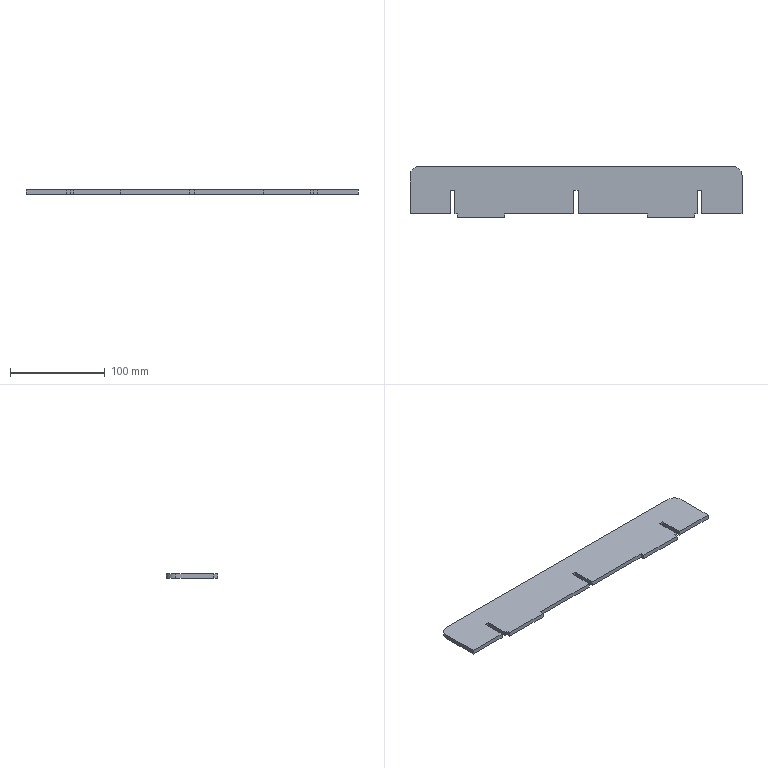Part | SolidWorks | features FlatPattern 1, SMBaseFlange 1, SheetMetal 1 | 1 solid | 28 faces | box 350 x 54 x 4.5 mm | volume 78838 mm3 | plane 26 | cylinder 2 | commonest cylinder face diameters 20 x2
STEP:
#1=CARTESIAN_POINT('',(-308.5,289.731,0.));
#2=VERTEX_POINT('',#1);
#3=CARTESIAN_POINT('',(-308.5,249.731,0.));
#4=VERTEX_POINT('',#3);
#5=CARTESIAN_POINT('',(-308.5,249.731,0.));
#6=DIRECTION('',(0.,-1.,0.));
#7=VECTOR('',#6,1000.);
#8=LINE('',#5,#7);
#9=EDGE_CURVE('',#2,#4,#8,.T.);
#10=ORIENTED_EDGE('',*,*,#9,.F.);
#11=CARTESIAN_POINT('',(-308.5,289.731,-4.5));
#12=VERTEX_POINT('',#11);
#13=CARTESIAN_POINT('',(-308.5,289.731,-4.5));
#14=DIRECTION('',(0.,0.,1.));
#15=VECTOR('',#14,1000.);
#16=LINE('',#13,#15);
#17=EDGE_CURVE('',#12,#2,#16,.T.);
#18=ORIENTED_EDGE('',*,*,#17,.F.);
#19=CARTESIAN_POINT('',(-308.5,249.731,-4.5));
#20=VERTEX_POINT('',#19);
#21=CARTESIAN_POINT('',(-308.5,249.731,-4.5));
#22=DIRECTION('',(0.,-1.,0.));
#23=VECTOR('',#22,1000.);
#24=LINE('',#21,#23);
#25=EDGE_CURVE('',#12,#20,#24,.T.);
#26=ORIENTED_EDGE('',*,*,#25,.T.);
#27=CARTESIAN_POINT('',(-308.5,249.731,-4.5));
#28=DIRECTION('',(0.,0.,1.));
#29=VECTOR('',#28,1000.);
#30=LINE('',#27,#29);
#31=EDGE_CURVE('',#20,#4,#30,.T.);
#32=ORIENTED_EDGE('',*,*,#31,.T.);
#33=EDGE_LOOP('',(#10,#18,#26,#32));
#34=FACE_OUTER_BOUND('',#33,.T.);
#35=CARTESIAN_POINT('',(-308.5,249.731,-4.5));
#36=DIRECTION('',(-1.,0.,0.));
#37=DIRECTION('',(0.,0.,1.));
#38=AXIS2_PLACEMENT_3D('',#35,#36,#37);
#39=PLANE('',#38);
#40=ADVANCED_FACE('',(#34),#39,.T.);
#41=CARTESIAN_POINT('',(-298.5,299.731,0.));
#42=VERTEX_POINT('',#41);
#43=CARTESIAN_POINT('',(-298.5,289.731,0.));
#44=DIRECTION('',(0.,0.,1.));
#45=DIRECTION('',(-1.,0.,0.));
#46=AXIS2_PLACEMENT_3D('',#43,#44,#45);
#47=CIRCLE('',#46,10.);
#48=EDGE_CURVE('',#42,#2,#47,.T.);
#49=ORIENTED_EDGE('',*,*,#48,.F.);
#50=CARTESIAN_POINT('',(-298.5,299.731,-4.5));
#51=VERTEX_POINT('',#50);
#52=CARTESIAN_POINT('',(-298.5,299.731,-4.5));
#53=DIRECTION('',(0.,0.,1.));
#54=VECTOR('',#53,1000.);
#55=LINE('',#52,#54);
#56=EDGE_CURVE('',#51,#42,#55,.T.);
#57=ORIENTED_EDGE('',*,*,#56,.F.);
#58=CARTESIAN_POINT('',(-298.5,289.731,-4.5));
#59=DIRECTION('',(0.,0.,1.));
#60=DIRECTION('',(-1.,0.,0.));
#61=AXIS2_PLACEMENT_3D('',#58,#59,#60);
#62=CIRCLE('',#61,10.);
#63=EDGE_CURVE('',#51,#12,#62,.T.);
#64=ORIENTED_EDGE('',*,*,#63,.T.);
#65=ORIENTED_EDGE('',*,*,#17,.T.);
#66=EDGE_LOOP('',(#49,#57,#64,#65));
#67=FACE_OUTER_BOUND('',#66,.T.);
#68=CARTESIAN_POINT('',(-298.5,289.731,-4.5));
#69=DIRECTION('',(0.,0.,1.));
#70=DIRECTION('',(1.,0.,0.));
#71=AXIS2_PLACEMENT_3D('',#68,#69,#70);
#72=CYLINDRICAL_SURFACE('',#71,10.);
#73=ADVANCED_FACE('',(#67),#72,.T.);
#74=CARTESIAN_POINT('',(31.5,299.731,0.));
#75=VERTEX_POINT('',#74);
#76=CARTESIAN_POINT('',(-298.5,299.731,0.));
#77=DIRECTION('',(-1.,0.,0.));
#78=VECTOR('',#77,1000.);
#79=LINE('',#76,#78);
#80=EDGE_CURVE('',#75,#42,#79,.T.);
#81=ORIENTED_EDGE('',*,*,#80,.F.);
#82=CARTESIAN_POINT('',(31.5,299.731,-4.5));
#83=VERTEX_POINT('',#82);
#84=CARTESIAN_POINT('',(31.5,299.731,-4.5));
#85=DIRECTION('',(0.,0.,1.));
#86=VECTOR('',#85,1000.);
#87=LINE('',#84,#86);
#88=EDGE_CURVE('',#83,#75,#87,.T.);
#89=ORIENTED_EDGE('',*,*,#88,.F.);
#90=CARTESIAN_POINT('',(-298.5,299.731,-4.5));
#91=DIRECTION('',(-1.,0.,0.));
#92=VECTOR('',#91,1000.);
#93=LINE('',#90,#92);
#94=EDGE_CURVE('',#83,#51,#93,.T.);
#95=ORIENTED_EDGE('',*,*,#94,.T.);
#96=ORIENTED_EDGE('',*,*,#56,.T.);
#97=EDGE_LOOP('',(#81,#89,#95,#96));
#98=FACE_OUTER_BOUND('',#97,.T.);
#99=CARTESIAN_POINT('',(-298.5,299.731,-4.5));
#100=DIRECTION('',(0.,1.,0.));
#101=DIRECTION('',(0.,0.,1.));
#102=AXIS2_PLACEMENT_3D('',#99,#100,#101);
#103=PLANE('',#102);
#104=ADVANCED_FACE('',(#98),#103,.T.);
#105=CARTESIAN_POINT('',(41.5,289.731,0.));
#106=VERTEX_POINT('',#105);
#107=CARTESIAN_POINT('',(31.5,289.731,0.));
#108=DIRECTION('',(0.,0.,1.));
#109=DIRECTION('',(-1.,0.,0.));
#110=AXIS2_PLACEMENT_3D('',#107,#108,#109);
#111=CIRCLE('',#110,10.);
#112=EDGE_CURVE('',#106,#75,#111,.T.);
#113=ORIENTED_EDGE('',*,*,#112,.F.);
#114=CARTESIAN_POINT('',(41.5,289.731,-4.5));
#115=VERTEX_POINT('',#114);
#116=CARTESIAN_POINT('',(41.5,289.731,-4.5));
#117=DIRECTION('',(0.,0.,1.));
#118=VECTOR('',#117,1000.);
#119=LINE('',#116,#118);
#120=EDGE_CURVE('',#115,#106,#119,.T.);
#121=ORIENTED_EDGE('',*,*,#120,.F.);
#122=CARTESIAN_POINT('',(31.5,289.731,-4.5));
#123=DIRECTION('',(0.,0.,1.));
#124=DIRECTION('',(-1.,0.,0.));
#125=AXIS2_PLACEMENT_3D('',#122,#123,#124);
#126=CIRCLE('',#125,10.);
#127=EDGE_CURVE('',#115,#83,#126,.T.);
#128=ORIENTED_EDGE('',*,*,#127,.T.);
#129=ORIENTED_EDGE('',*,*,#88,.T.);
#130=EDGE_LOOP('',(#113,#121,#128,#129));
#131=FACE_OUTER_BOUND('',#130,.T.);
#132=CARTESIAN_POINT('',(31.5,289.731,-4.5));
#133=DIRECTION('',(0.,0.,1.));
#134=DIRECTION('',(1.,0.,0.));
#135=AXIS2_PLACEMENT_3D('',#132,#133,#134);
#136=CYLINDRICAL_SURFACE('',#135,10.);
#137=ADVANCED_FACE('',(#131),#136,.T.);
#138=CARTESIAN_POINT('',(41.5,249.731,0.));
#139=VERTEX_POINT('',#138);
#140=CARTESIAN_POINT('',(41.5,249.731,0.));
#141=DIRECTION('',(0.,1.,0.));
#142=VECTOR('',#141,1000.);
#143=LINE('',#140,#142);
#144=EDGE_CURVE('',#139,#106,#143,.T.);
#145=ORIENTED_EDGE('',*,*,#144,.F.);
#146=CARTESIAN_POINT('',(41.5,249.731,-4.5));
#147=VERTEX_POINT('',#146);
#148=CARTESIAN_POINT('',(41.5,249.731,-4.5));
#149=DIRECTION('',(0.,0.,1.));
#150=VECTOR('',#149,1000.);
#151=LINE('',#148,#150);
#152=EDGE_CURVE('',#147,#139,#151,.T.);
#153=ORIENTED_EDGE('',*,*,#152,.F.);
#154=CARTESIAN_POINT('',(41.5,249.731,-4.5));
#155=DIRECTION('',(0.,1.,0.));
#156=VECTOR('',#155,1000.);
#157=LINE('',#154,#156);
#158=EDGE_CURVE('',#147,#115,#157,.T.);
#159=ORIENTED_EDGE('',*,*,#158,.T.);
#160=ORIENTED_EDGE('',*,*,#120,.T.);
#161=EDGE_LOOP('',(#145,#153,#159,#160));
#162=FACE_OUTER_BOUND('',#161,.T.);
#163=CARTESIAN_POINT('',(41.5,249.731,-4.5));
#164=DIRECTION('',(1.,0.,0.));
#165=DIRECTION('',(0.,0.,-1.));
#166=AXIS2_PLACEMENT_3D('',#163,#164,#165);
#167=PLANE('',#166);
#168=ADVANCED_FACE('',(#162),#167,.T.);
#169=CARTESIAN_POINT('',(-1.25,249.731,0.));
#170=VERTEX_POINT('',#169);
#171=CARTESIAN_POINT('',(-1.25,249.731,0.));
#172=DIRECTION('',(1.,0.,0.));
#173=VECTOR('',#172,1000.);
#174=LINE('',#171,#173);
#175=EDGE_CURVE('',#170,#139,#174,.T.);
#176=ORIENTED_EDGE('',*,*,#175,.F.);
#177=CARTESIAN_POINT('',(-1.25,249.731,-4.5));
#178=VERTEX_POINT('',#177);
#179=CARTESIAN_POINT('',(-1.25,249.731,-4.5));
#180=DIRECTION('',(0.,0.,1.));
#181=VECTOR('',#180,1000.);
#182=LINE('',#179,#181);
#183=EDGE_CURVE('',#178,#170,#182,.T.);
#184=ORIENTED_EDGE('',*,*,#183,.F.);
#185=CARTESIAN_POINT('',(-1.25,249.731,-4.5));
#186=DIRECTION('',(1.,0.,0.));
#187=VECTOR('',#186,1000.);
#188=LINE('',#185,#187);
#189=EDGE_CURVE('',#178,#147,#188,.T.);
#190=ORIENTED_EDGE('',*,*,#189,.T.);
#191=ORIENTED_EDGE('',*,*,#152,.T.);
#192=EDGE_LOOP('',(#176,#184,#190,#191));
#193=FACE_OUTER_BOUND('',#192,.T.);
#194=CARTESIAN_POINT('',(-1.25,249.731,-4.5));
#195=DIRECTION('',(0.,-1.,0.));
#196=DIRECTION('',(0.,0.,-1.));
#197=AXIS2_PLACEMENT_3D('',#194,#195,#196);
#198=PLANE('',#197);
#199=ADVANCED_FACE('',(#193),#198,.T.);
#200=CARTESIAN_POINT('',(-1.25,274.731,0.));
#201=VERTEX_POINT('',#200);
#202=CARTESIAN_POINT('',(-1.25,274.731,0.));
#203=DIRECTION('',(0.,-1.,0.));
#204=VECTOR('',#203,1000.);
#205=LINE('',#202,#204);
#206=EDGE_CURVE('',#201,#170,#205,.T.);
#207=ORIENTED_EDGE('',*,*,#206,.F.);
#208=CARTESIAN_POINT('',(-1.25,274.731,-4.5));
#209=VERTEX_POINT('',#208);
#210=CARTESIAN_POINT('',(-1.25,274.731,-4.5));
#211=DIRECTION('',(0.,0.,1.));
#212=VECTOR('',#211,1000.);
#213=LINE('',#210,#212);
#214=EDGE_CURVE('',#209,#201,#213,.T.);
#215=ORIENTED_EDGE('',*,*,#214,.F.);
#216=CARTESIAN_POINT('',(-1.25,274.731,-4.5));
#217=DIRECTION('',(0.,-1.,0.));
#218=VECTOR('',#217,1000.);
#219=LINE('',#216,#218);
#220=EDGE_CURVE('',#209,#178,#219,.T.);
#221=ORIENTED_EDGE('',*,*,#220,.T.);
#222=ORIENTED_EDGE('',*,*,#183,.T.);
#223=EDGE_LOOP('',(#207,#215,#221,#222));
#224=FACE_OUTER_BOUND('',#223,.T.);
#225=CARTESIAN_POINT('',(-1.25,274.731,-4.5));
#226=DIRECTION('',(-1.,0.,0.));
#227=DIRECTION('',(0.,-1.,0.));
#228=AXIS2_PLACEMENT_3D('',#225,#226,#227);
#229=PLANE('',#228);
#230=ADVANCED_FACE('',(#224),#229,.T.);
#231=CARTESIAN_POINT('',(-5.75,274.731,0.));
#232=VERTEX_POINT('',#231);
#233=CARTESIAN_POINT('',(-5.75,274.731,0.));
#234=DIRECTION('',(1.,0.,0.));
#235=VECTOR('',#234,1000.);
#236=LINE('',#233,#235);
#237=EDGE_CURVE('',#232,#201,#236,.T.);
#238=ORIENTED_EDGE('',*,*,#237,.F.);
#239=CARTESIAN_POINT('',(-5.75,274.731,-4.5));
#240=VERTEX_POINT('',#239);
#241=CARTESIAN_POINT('',(-5.75,274.731,-4.5));
#242=DIRECTION('',(0.,0.,1.));
#243=VECTOR('',#242,1000.);
#244=LINE('',#241,#243);
#245=EDGE_CURVE('',#240,#232,#244,.T.);
#246=ORIENTED_EDGE('',*,*,#245,.F.);
#247=CARTESIAN_POINT('',(-5.75,274.731,-4.5));
#248=DIRECTION('',(1.,0.,0.));
#249=VECTOR('',#248,1000.);
#250=LINE('',#247,#249);
#251=EDGE_CURVE('',#240,#209,#250,.T.);
#252=ORIENTED_EDGE('',*,*,#251,.T.);
#253=ORIENTED_EDGE('',*,*,#214,.T.);
#254=EDGE_LOOP('',(#238,#246,#252,#253));
#255=FACE_OUTER_BOUND('',#254,.T.);
#256=CARTESIAN_POINT('',(-5.75,274.731,-4.5));
#257=DIRECTION('',(0.,-1.,0.));
#258=DIRECTION('',(0.,0.,-1.));
#259=AXIS2_PLACEMENT_3D('',#256,#257,#258);
#260=PLANE('',#259);
#261=ADVANCED_FACE('',(#255),#260,.T.);
#262=CARTESIAN_POINT('',(-5.75,249.731,0.));
#263=VERTEX_POINT('',#262);
#264=CARTESIAN_POINT('',(-5.75,249.731,0.));
#265=DIRECTION('',(0.,1.,0.));
#266=VECTOR('',#265,1000.);
#267=LINE('',#264,#266);
#268=EDGE_CURVE('',#263,#232,#267,.T.);
#269=ORIENTED_EDGE('',*,*,#268,.F.);
#270=CARTESIAN_POINT('',(-5.75,249.731,-4.5));
#271=VERTEX_POINT('',#270);
#272=CARTESIAN_POINT('',(-5.75,249.731,-4.5));
#273=DIRECTION('',(0.,0.,1.));
#274=VECTOR('',#273,1000.);
#275=LINE('',#272,#274);
#276=EDGE_CURVE('',#271,#263,#275,.T.);
#277=ORIENTED_EDGE('',*,*,#276,.F.);
#278=CARTESIAN_POINT('',(-5.75,249.731,-4.5));
#279=DIRECTION('',(0.,1.,0.));
#280=VECTOR('',#279,1000.);
#281=LINE('',#278,#280);
#282=EDGE_CURVE('',#271,#240,#281,.T.);
#283=ORIENTED_EDGE('',*,*,#282,.T.);
#284=ORIENTED_EDGE('',*,*,#245,.T.);
#285=EDGE_LOOP('',(#269,#277,#283,#284));
#286=FACE_OUTER_BOUND('',#285,.T.);
#287=CARTESIAN_POINT('',(-5.75,249.731,-4.5));
#288=DIRECTION('',(1.,0.,0.));
#289=DIRECTION('',(0.,1.,0.));
#290=AXIS2_PLACEMENT_3D('',#287,#288,#289);
#291=PLANE('',#290);
#292=ADVANCED_FACE('',(#286),#291,.T.);
#293=CARTESIAN_POINT('',(-8.5,249.731,0.));
#294=VERTEX_POINT('',#293);
#295=CARTESIAN_POINT('',(-8.5,249.731,0.));
#296=DIRECTION('',(1.,0.,0.));
#297=VECTOR('',#296,1000.);
#298=LINE('',#295,#297);
#299=EDGE_CURVE('',#294,#263,#298,.T.);
#300=ORIENTED_EDGE('',*,*,#299,.F.);
#301=CARTESIAN_POINT('',(-8.5,249.731,-4.5));
#302=VERTEX_POINT('',#301);
#303=CARTESIAN_POINT('',(-8.5,249.731,-4.5));
#304=DIRECTION('',(0.,0.,1.));
#305=VECTOR('',#304,1000.);
#306=LINE('',#303,#305);
#307=EDGE_CURVE('',#302,#294,#306,.T.);
#308=ORIENTED_EDGE('',*,*,#307,.F.);
#309=CARTESIAN_POINT('',(-8.5,249.731,-4.5));
#310=DIRECTION('',(1.,0.,0.));
#311=VECTOR('',#310,1000.);
#312=LINE('',#309,#311);
#313=EDGE_CURVE('',#302,#271,#312,.T.);
#314=ORIENTED_EDGE('',*,*,#313,.T.);
#315=ORIENTED_EDGE('',*,*,#276,.T.);
#316=EDGE_LOOP('',(#300,#308,#314,#315));
#317=FACE_OUTER_BOUND('',#316,.T.);
#318=CARTESIAN_POINT('',(-8.5,249.731,-4.5));
#319=DIRECTION('',(0.,-1.,0.));
#320=DIRECTION('',(1.,0.,0.));
#321=AXIS2_PLACEMENT_3D('',#318,#319,#320);
#322=PLANE('',#321);
#323=ADVANCED_FACE('',(#317),#322,.T.);
#324=CARTESIAN_POINT('',(-8.5,245.731,0.));
#325=VERTEX_POINT('',#324);
#326=CARTESIAN_POINT('',(-8.5,249.731,0.));
#327=DIRECTION('',(0.,1.,0.));
#328=VECTOR('',#327,1000.);
#329=LINE('',#326,#328);
#330=EDGE_CURVE('',#325,#294,#329,.T.);
#331=ORIENTED_EDGE('',*,*,#330,.F.);
#332=CARTESIAN_POINT('',(-8.5,245.731,-4.5));
#333=VERTEX_POINT('',#332);
#334=CARTESIAN_POINT('',(-8.5,245.731,-4.5));
#335=DIRECTION('',(0.,0.,1.));
#336=VECTOR('',#335,1000.);
#337=LINE('',#334,#336);
#338=EDGE_CURVE('',#333,#325,#337,.T.);
#339=ORIENTED_EDGE('',*,*,#338,.F.);
#340=CARTESIAN_POINT('',(-8.5,249.731,-4.5));
#341=DIRECTION('',(0.,1.,0.));
#342=VECTOR('',#341,1000.);
#343=LINE('',#340,#342);
#344=EDGE_CURVE('',#333,#302,#343,.T.);
#345=ORIENTED_EDGE('',*,*,#344,.T.);
#346=ORIENTED_EDGE('',*,*,#307,.T.);
#347=EDGE_LOOP('',(#331,#339,#345,#346));
#348=FACE_OUTER_BOUND('',#347,.T.);
#349=CARTESIAN_POINT('',(-8.5,249.731,-4.5));
#350=DIRECTION('',(1.,0.,0.));
#351=DIRECTION('',(0.,0.,-1.));
#352=AXIS2_PLACEMENT_3D('',#349,#350,#351);
#353=PLANE('',#352);
#354=ADVANCED_FACE('',(#348),#353,.T.);
#355=CARTESIAN_POINT('',(-58.5,245.731,0.));
#356=VERTEX_POINT('',#355);
#357=CARTESIAN_POINT('',(-8.5,245.731,0.));
#358=DIRECTION('',(1.,0.,0.));
#359=VECTOR('',#358,1000.);
#360=LINE('',#357,#359);
#361=EDGE_CURVE('',#356,#325,#360,.T.);
#362=ORIENTED_EDGE('',*,*,#361,.F.);
#363=CARTESIAN_POINT('',(-58.5,245.731,-4.5));
#364=VERTEX_POINT('',#363);
#365=CARTESIAN_POINT('',(-58.5,245.731,-4.5));
#366=DIRECTION('',(0.,0.,1.));
#367=VECTOR('',#366,1000.);
#368=LINE('',#365,#367);
#369=EDGE_CURVE('',#364,#356,#368,.T.);
#370=ORIENTED_EDGE('',*,*,#369,.F.);
#371=CARTESIAN_POINT('',(-8.5,245.731,-4.5));
#372=DIRECTION('',(1.,0.,0.));
#373=VECTOR('',#372,1000.);
#374=LINE('',#371,#373);
#375=EDGE_CURVE('',#364,#333,#374,.T.);
#376=ORIENTED_EDGE('',*,*,#375,.T.);
#377=ORIENTED_EDGE('',*,*,#338,.T.);
#378=EDGE_LOOP('',(#362,#370,#376,#377));
#379=FACE_OUTER_BOUND('',#378,.T.);
#380=CARTESIAN_POINT('',(-8.5,245.731,-4.5));
#381=DIRECTION('',(0.,-1.,0.));
#382=DIRECTION('',(0.,0.,-1.));
#383=AXIS2_PLACEMENT_3D('',#380,#381,#382);
#384=PLANE('',#383);
#385=ADVANCED_FACE('',(#379),#384,.T.);
#386=CARTESIAN_POINT('',(-58.5,249.731,0.));
#387=VERTEX_POINT('',#386);
#388=CARTESIAN_POINT('',(-58.5,245.731,0.));
#389=DIRECTION('',(0.,-1.,0.));
#390=VECTOR('',#389,1000.);
#391=LINE('',#388,#390);
#392=EDGE_CURVE('',#387,#356,#391,.T.);
#393=ORIENTED_EDGE('',*,*,#392,.F.);
#394=CARTESIAN_POINT('',(-58.5,249.731,-4.5));
#395=VERTEX_POINT('',#394);
#396=CARTESIAN_POINT('',(-58.5,249.731,-4.5));
#397=DIRECTION('',(0.,0.,1.));
#398=VECTOR('',#397,1000.);
#399=LINE('',#396,#398);
#400=EDGE_CURVE('',#395,#387,#399,.T.);
#401=ORIENTED_EDGE('',*,*,#400,.F.);
#402=CARTESIAN_POINT('',(-58.5,245.731,-4.5));
#403=DIRECTION('',(0.,-1.,0.));
#404=VECTOR('',#403,1000.);
#405=LINE('',#402,#404);
#406=EDGE_CURVE('',#395,#364,#405,.T.);
#407=ORIENTED_EDGE('',*,*,#406,.T.);
#408=ORIENTED_EDGE('',*,*,#369,.T.);
#409=EDGE_LOOP('',(#393,#401,#407,#408));
#410=FACE_OUTER_BOUND('',#409,.T.);
#411=CARTESIAN_POINT('',(-58.5,245.731,-4.5));
#412=DIRECTION('',(-1.,0.,0.));
#413=DIRECTION('',(0.,0.,1.));
#414=AXIS2_PLACEMENT_3D('',#411,#412,#413);
#415=PLANE('',#414);
#416=ADVANCED_FACE('',(#410),#415,.T.);
#417=CARTESIAN_POINT('',(-131.25,249.731,0.));
#418=VERTEX_POINT('',#417);
#419=CARTESIAN_POINT('',(-131.25,249.731,0.));
#420=DIRECTION('',(1.,0.,0.));
#421=VECTOR('',#420,1000.);
#422=LINE('',#419,#421);
#423=EDGE_CURVE('',#418,#387,#422,.T.);
#424=ORIENTED_EDGE('',*,*,#423,.F.);
#425=CARTESIAN_POINT('',(-131.25,249.731,-4.5));
#426=VERTEX_POINT('',#425);
#427=CARTESIAN_POINT('',(-131.25,249.731,-4.5));
#428=DIRECTION('',(0.,0.,1.));
#429=VECTOR('',#428,1000.);
#430=LINE('',#427,#429);
#431=EDGE_CURVE('',#426,#418,#430,.T.);
#432=ORIENTED_EDGE('',*,*,#431,.F.);
#433=CARTESIAN_POINT('',(-131.25,249.731,-4.5));
#434=DIRECTION('',(1.,0.,0.));
#435=VECTOR('',#434,1000.);
#436=LINE('',#433,#435);
#437=EDGE_CURVE('',#426,#395,#436,.T.);
#438=ORIENTED_EDGE('',*,*,#437,.T.);
#439=ORIENTED_EDGE('',*,*,#400,.T.);
#440=EDGE_LOOP('',(#424,#432,#438,#439));
#441=FACE_OUTER_BOUND('',#440,.T.);
#442=CARTESIAN_POINT('',(-131.25,249.731,-4.5));
#443=DIRECTION('',(0.,-1.,0.));
#444=DIRECTION('',(1.,0.,0.));
#445=AXIS2_PLACEMENT_3D('',#442,#443,#444);
#446=PLANE('',#445);
#447=ADVANCED_FACE('',(#441),#446,.T.);
#448=CARTESIAN_POINT('',(-131.25,274.731,0.));
#449=VERTEX_POINT('',#448);
#450=CARTESIAN_POINT('',(-131.25,274.731,0.));
#451=DIRECTION('',(0.,-1.,0.));
#452=VECTOR('',#451,1000.);
#453=LINE('',#450,#452);
#454=EDGE_CURVE('',#449,#418,#453,.T.);
#455=ORIENTED_EDGE('',*,*,#454,.F.);
#456=CARTESIAN_POINT('',(-131.25,274.731,-4.5));
#457=VERTEX_POINT('',#456);
#458=CARTESIAN_POINT('',(-131.25,274.731,-4.5));
#459=DIRECTION('',(0.,0.,1.));
#460=VECTOR('',#459,1000.);
#461=LINE('',#458,#460);
#462=EDGE_CURVE('',#457,#449,#461,.T.);
#463=ORIENTED_EDGE('',*,*,#462,.F.);
#464=CARTESIAN_POINT('',(-131.25,274.731,-4.5));
#465=DIRECTION('',(0.,-1.,0.));
#466=VECTOR('',#465,1000.);
#467=LINE('',#464,#466);
#468=EDGE_CURVE('',#457,#426,#467,.T.);
#469=ORIENTED_EDGE('',*,*,#468,.T.);
#470=ORIENTED_EDGE('',*,*,#431,.T.);
#471=EDGE_LOOP('',(#455,#463,#469,#470));
#472=FACE_OUTER_BOUND('',#471,.T.);
#473=CARTESIAN_POINT('',(-131.25,274.731,-4.5));
#474=DIRECTION('',(-1.,0.,0.));
#475=DIRECTION('',(0.,-1.,0.));
#476=AXIS2_PLACEMENT_3D('',#473,#474,#475);
#477=PLANE('',#476);
#478=ADVANCED_FACE('',(#472),#477,.T.);
#479=CARTESIAN_POINT('',(-135.75,274.731,0.));
#480=VERTEX_POINT('',#479);
#481=CARTESIAN_POINT('',(-135.75,274.731,0.));
#482=DIRECTION('',(1.,0.,0.));
#483=VECTOR('',#482,1000.);
#484=LINE('',#481,#483);
#485=EDGE_CURVE('',#480,#449,#484,.T.);
#486=ORIENTED_EDGE('',*,*,#485,.F.);
#487=CARTESIAN_POINT('',(-135.75,274.731,-4.5));
#488=VERTEX_POINT('',#487);
#489=CARTESIAN_POINT('',(-135.75,274.731,-4.5));
#490=DIRECTION('',(0.,0.,1.));
#491=VECTOR('',#490,1000.);
#492=LINE('',#489,#491);
#493=EDGE_CURVE('',#488,#480,#492,.T.);
#494=ORIENTED_EDGE('',*,*,#493,.F.);
#495=CARTESIAN_POINT('',(-135.75,274.731,-4.5));
#496=DIRECTION('',(1.,0.,0.));
#497=VECTOR('',#496,1000.);
#498=LINE('',#495,#497);
#499=EDGE_CURVE('',#488,#457,#498,.T.);
#500=ORIENTED_EDGE('',*,*,#499,.T.);
#501=ORIENTED_EDGE('',*,*,#462,.T.);
#502=EDGE_LOOP('',(#486,#494,#500,#501));
#503=FACE_OUTER_BOUND('',#502,.T.);
#504=CARTESIAN_POINT('',(-135.75,274.731,-4.5));
#505=DIRECTION('',(0.,-1.,0.));
#506=DIRECTION('',(0.,0.,-1.));
#507=AXIS2_PLACEMENT_3D('',#504,#505,#506);
#508=PLANE('',#507);
#509=ADVANCED_FACE('',(#503),#508,.T.);
#510=CARTESIAN_POINT('',(-135.75,249.731,0.));
#511=VERTEX_POINT('',#510);
#512=CARTESIAN_POINT('',(-135.75,249.731,0.));
#513=DIRECTION('',(0.,1.,0.));
#514=VECTOR('',#513,1000.);
#515=LINE('',#512,#514);
#516=EDGE_CURVE('',#511,#480,#515,.T.);
#517=ORIENTED_EDGE('',*,*,#516,.F.);
#518=CARTESIAN_POINT('',(-135.75,249.731,-4.5));
#519=VERTEX_POINT('',#518);
#520=CARTESIAN_POINT('',(-135.75,249.731,-4.5));
#521=DIRECTION('',(0.,0.,1.));
#522=VECTOR('',#521,1000.);
#523=LINE('',#520,#522);
#524=EDGE_CURVE('',#519,#511,#523,.T.);
#525=ORIENTED_EDGE('',*,*,#524,.F.);
#526=CARTESIAN_POINT('',(-135.75,249.731,-4.5));
#527=DIRECTION('',(0.,1.,0.));
#528=VECTOR('',#527,1000.);
#529=LINE('',#526,#528);
#530=EDGE_CURVE('',#519,#488,#529,.T.);
#531=ORIENTED_EDGE('',*,*,#530,.T.);
#532=ORIENTED_EDGE('',*,*,#493,.T.);
#533=EDGE_LOOP('',(#517,#525,#531,#532));
#534=FACE_OUTER_BOUND('',#533,.T.);
#535=CARTESIAN_POINT('',(-135.75,249.731,-4.5));
#536=DIRECTION('',(1.,0.,0.));
#537=DIRECTION('',(0.,1.,0.));
#538=AXIS2_PLACEMENT_3D('',#535,#536,#537);
#539=PLANE('',#538);
#540=ADVANCED_FACE('',(#534),#539,.T.);
#541=CARTESIAN_POINT('',(-208.5,249.731,0.));
#542=VERTEX_POINT('',#541);
#543=CARTESIAN_POINT('',(-208.5,249.731,0.));
#544=DIRECTION('',(1.,0.,0.));
#545=VECTOR('',#544,1000.);
#546=LINE('',#543,#545);
#547=EDGE_CURVE('',#542,#511,#546,.T.);
#548=ORIENTED_EDGE('',*,*,#547,.F.);
#549=CARTESIAN_POINT('',(-208.5,249.731,-4.5));
#550=VERTEX_POINT('',#549);
#551=CARTESIAN_POINT('',(-208.5,249.731,-4.5));
#552=DIRECTION('',(0.,0.,1.));
#553=VECTOR('',#552,1000.);
#554=LINE('',#551,#553);
#555=EDGE_CURVE('',#550,#542,#554,.T.);
#556=ORIENTED_EDGE('',*,*,#555,.F.);
#557=CARTESIAN_POINT('',(-208.5,249.731,-4.5));
#558=DIRECTION('',(1.,0.,0.));
#559=VECTOR('',#558,1000.);
#560=LINE('',#557,#559);
#561=EDGE_CURVE('',#550,#519,#560,.T.);
#562=ORIENTED_EDGE('',*,*,#561,.T.);
#563=ORIENTED_EDGE('',*,*,#524,.T.);
#564=EDGE_LOOP('',(#548,#556,#562,#563));
#565=FACE_OUTER_BOUND('',#564,.T.);
#566=CARTESIAN_POINT('',(-208.5,249.731,-4.5));
#567=DIRECTION('',(0.,-1.,0.));
#568=DIRECTION('',(1.,0.,0.));
#569=AXIS2_PLACEMENT_3D('',#566,#567,#568);
#570=PLANE('',#569);
#571=ADVANCED_FACE('',(#565),#570,.T.);
#572=CARTESIAN_POINT('',(-208.5,245.731,0.));
#573=VERTEX_POINT('',#572);
#574=CARTESIAN_POINT('',(-208.5,245.731,0.));
#575=DIRECTION('',(0.,1.,0.));
#576=VECTOR('',#575,1000.);
#577=LINE('',#574,#576);
#578=EDGE_CURVE('',#573,#542,#577,.T.);
#579=ORIENTED_EDGE('',*,*,#578,.F.);
#580=CARTESIAN_POINT('',(-208.5,245.731,-4.5));
#581=VERTEX_POINT('',#580);
#582=CARTESIAN_POINT('',(-208.5,245.731,-4.5));
#583=DIRECTION('',(0.,0.,1.));
#584=VECTOR('',#583,1000.);
#585=LINE('',#582,#584);
#586=EDGE_CURVE('',#581,#573,#585,.T.);
#587=ORIENTED_EDGE('',*,*,#586,.F.);
#588=CARTESIAN_POINT('',(-208.5,245.731,-4.5));
#589=DIRECTION('',(0.,1.,0.));
#590=VECTOR('',#589,1000.);
#591=LINE('',#588,#590);
#592=EDGE_CURVE('',#581,#550,#591,.T.);
#593=ORIENTED_EDGE('',*,*,#592,.T.);
#594=ORIENTED_EDGE('',*,*,#555,.T.);
#595=EDGE_LOOP('',(#579,#587,#593,#594));
#596=FACE_OUTER_BOUND('',#595,.T.);
#597=CARTESIAN_POINT('',(-208.5,245.731,-4.5));
#598=DIRECTION('',(1.,0.,0.));
#599=DIRECTION('',(0.,0.,-1.));
#600=AXIS2_PLACEMENT_3D('',#597,#598,#599);
#601=PLANE('',#600);
#602=ADVANCED_FACE('',(#596),#601,.T.);
#603=CARTESIAN_POINT('',(-258.5,245.731,0.));
#604=VERTEX_POINT('',#603);
#605=CARTESIAN_POINT('',(-258.5,245.731,0.));
#606=DIRECTION('',(1.,0.,0.));
#607=VECTOR('',#606,1000.);
#608=LINE('',#605,#607);
#609=EDGE_CURVE('',#604,#573,#608,.T.);
#610=ORIENTED_EDGE('',*,*,#609,.F.);
#611=CARTESIAN_POINT('',(-258.5,245.731,-4.5));
#612=VERTEX_POINT('',#611);
#613=CARTESIAN_POINT('',(-258.5,245.731,-4.5));
#614=DIRECTION('',(0.,0.,1.));
#615=VECTOR('',#614,1000.);
#616=LINE('',#613,#615);
#617=EDGE_CURVE('',#612,#604,#616,.T.);
#618=ORIENTED_EDGE('',*,*,#617,.F.);
#619=CARTESIAN_POINT('',(-258.5,245.731,-4.5));
#620=DIRECTION('',(1.,0.,0.));
#621=VECTOR('',#620,1000.);
#622=LINE('',#619,#621);
#623=EDGE_CURVE('',#612,#581,#622,.T.);
#624=ORIENTED_EDGE('',*,*,#623,.T.);
#625=ORIENTED_EDGE('',*,*,#586,.T.);
#626=EDGE_LOOP('',(#610,#618,#624,#625));
#627=FACE_OUTER_BOUND('',#626,.T.);
#628=CARTESIAN_POINT('',(-258.5,245.731,-4.5));
#629=DIRECTION('',(0.,-1.,0.));
#630=DIRECTION('',(0.,0.,-1.));
#631=AXIS2_PLACEMENT_3D('',#628,#629,#630);
#632=PLANE('',#631);
#633=ADVANCED_FACE('',(#627),#632,.T.);
#634=CARTESIAN_POINT('',(-258.5,249.731,0.));
#635=VERTEX_POINT('',#634);
#636=CARTESIAN_POINT('',(-258.5,249.731,0.));
#637=DIRECTION('',(0.,-1.,0.));
#638=VECTOR('',#637,1000.);
#639=LINE('',#636,#638);
#640=EDGE_CURVE('',#635,#604,#639,.T.);
#641=ORIENTED_EDGE('',*,*,#640,.F.);
#642=CARTESIAN_POINT('',(-258.5,249.731,-4.5));
#643=VERTEX_POINT('',#642);
#644=CARTESIAN_POINT('',(-258.5,249.731,-4.5));
#645=DIRECTION('',(0.,0.,1.));
#646=VECTOR('',#645,1000.);
#647=LINE('',#644,#646);
#648=EDGE_CURVE('',#643,#635,#647,.T.);
#649=ORIENTED_EDGE('',*,*,#648,.F.);
#650=CARTESIAN_POINT('',(-258.5,249.731,-4.5));
#651=DIRECTION('',(0.,-1.,0.));
#652=VECTOR('',#651,1000.);
#653=LINE('',#650,#652);
#654=EDGE_CURVE('',#643,#612,#653,.T.);
#655=ORIENTED_EDGE('',*,*,#654,.T.);
#656=ORIENTED_EDGE('',*,*,#617,.T.);
#657=EDGE_LOOP('',(#641,#649,#655,#656));
#658=FACE_OUTER_BOUND('',#657,.T.);
#659=CARTESIAN_POINT('',(-258.5,249.731,-4.5));
#660=DIRECTION('',(-1.,0.,0.));
#661=DIRECTION('',(0.,0.,1.));
#662=AXIS2_PLACEMENT_3D('',#659,#660,#661);
#663=PLANE('',#662);
#664=ADVANCED_FACE('',(#658),#663,.T.);
#665=CARTESIAN_POINT('',(-261.25,249.731,0.));
#666=VERTEX_POINT('',#665);
#667=CARTESIAN_POINT('',(-261.25,249.731,0.));
#668=DIRECTION('',(1.,0.,0.));
#669=VECTOR('',#668,1000.);
#670=LINE('',#667,#669);
#671=EDGE_CURVE('',#666,#635,#670,.T.);
#672=ORIENTED_EDGE('',*,*,#671,.F.);
#673=CARTESIAN_POINT('',(-261.25,249.731,-4.5));
#674=VERTEX_POINT('',#673);
#675=CARTESIAN_POINT('',(-261.25,249.731,-4.5));
#676=DIRECTION('',(0.,0.,1.));
#677=VECTOR('',#676,1000.);
#678=LINE('',#675,#677);
#679=EDGE_CURVE('',#674,#666,#678,.T.);
#680=ORIENTED_EDGE('',*,*,#679,.F.);
#681=CARTESIAN_POINT('',(-261.25,249.731,-4.5));
#682=DIRECTION('',(1.,0.,0.));
#683=VECTOR('',#682,1000.);
#684=LINE('',#681,#683);
#685=EDGE_CURVE('',#674,#643,#684,.T.);
#686=ORIENTED_EDGE('',*,*,#685,.T.);
#687=ORIENTED_EDGE('',*,*,#648,.T.);
#688=EDGE_LOOP('',(#672,#680,#686,#687));
#689=FACE_OUTER_BOUND('',#688,.T.);
#690=CARTESIAN_POINT('',(-261.25,249.731,-4.5));
#691=DIRECTION('',(0.,-1.,0.));
#692=DIRECTION('',(1.,0.,0.));
#693=AXIS2_PLACEMENT_3D('',#690,#691,#692);
#694=PLANE('',#693);
#695=ADVANCED_FACE('',(#689),#694,.T.);
#696=CARTESIAN_POINT('',(-261.25,274.731,0.));
#697=VERTEX_POINT('',#696);
#698=CARTESIAN_POINT('',(-261.25,274.731,0.));
#699=DIRECTION('',(0.,-1.,0.));
#700=VECTOR('',#699,1000.);
#701=LINE('',#698,#700);
#702=EDGE_CURVE('',#697,#666,#701,.T.);
#703=ORIENTED_EDGE('',*,*,#702,.F.);
#704=CARTESIAN_POINT('',(-261.25,274.731,-4.5));
#705=VERTEX_POINT('',#704);
#706=CARTESIAN_POINT('',(-261.25,274.731,-4.5));
#707=DIRECTION('',(0.,0.,1.));
#708=VECTOR('',#707,1000.);
#709=LINE('',#706,#708);
#710=EDGE_CURVE('',#705,#697,#709,.T.);
#711=ORIENTED_EDGE('',*,*,#710,.F.);
#712=CARTESIAN_POINT('',(-261.25,274.731,-4.5));
#713=DIRECTION('',(0.,-1.,0.));
#714=VECTOR('',#713,1000.);
#715=LINE('',#712,#714);
#716=EDGE_CURVE('',#705,#674,#715,.T.);
#717=ORIENTED_EDGE('',*,*,#716,.T.);
#718=ORIENTED_EDGE('',*,*,#679,.T.);
#719=EDGE_LOOP('',(#703,#711,#717,#718));
#720=FACE_OUTER_BOUND('',#719,.T.);
#721=CARTESIAN_POINT('',(-261.25,274.731,-4.5));
#722=DIRECTION('',(-1.,0.,0.));
#723=DIRECTION('',(0.,-1.,0.));
#724=AXIS2_PLACEMENT_3D('',#721,#722,#723);
#725=PLANE('',#724);
#726=ADVANCED_FACE('',(#720),#725,.T.);
#727=CARTESIAN_POINT('',(-265.75,274.731,0.));
#728=VERTEX_POINT('',#727);
#729=CARTESIAN_POINT('',(-265.75,274.731,0.));
#730=DIRECTION('',(1.,0.,0.));
#731=VECTOR('',#730,1000.);
#732=LINE('',#729,#731);
#733=EDGE_CURVE('',#728,#697,#732,.T.);
#734=ORIENTED_EDGE('',*,*,#733,.F.);
#735=CARTESIAN_POINT('',(-265.75,274.731,-4.5));
#736=VERTEX_POINT('',#735);
#737=CARTESIAN_POINT('',(-265.75,274.731,-4.5));
#738=DIRECTION('',(0.,0.,1.));
#739=VECTOR('',#738,1000.);
#740=LINE('',#737,#739);
#741=EDGE_CURVE('',#736,#728,#740,.T.);
#742=ORIENTED_EDGE('',*,*,#741,.F.);
#743=CARTESIAN_POINT('',(-265.75,274.731,-4.5));
#744=DIRECTION('',(1.,0.,0.));
#745=VECTOR('',#744,1000.);
#746=LINE('',#743,#745);
#747=EDGE_CURVE('',#736,#705,#746,.T.);
#748=ORIENTED_EDGE('',*,*,#747,.T.);
#749=ORIENTED_EDGE('',*,*,#710,.T.);
#750=EDGE_LOOP('',(#734,#742,#748,#749));
#751=FACE_OUTER_BOUND('',#750,.T.);
#752=CARTESIAN_POINT('',(-265.75,274.731,-4.5));
#753=DIRECTION('',(0.,-1.,0.));
#754=DIRECTION('',(0.,0.,-1.));
#755=AXIS2_PLACEMENT_3D('',#752,#753,#754);
#756=PLANE('',#755);
#757=ADVANCED_FACE('',(#751),#756,.T.);
#758=CARTESIAN_POINT('',(-265.75,249.731,0.));
#759=VERTEX_POINT('',#758);
#760=CARTESIAN_POINT('',(-265.75,249.731,0.));
#761=DIRECTION('',(0.,1.,0.));
#762=VECTOR('',#761,1000.);
#763=LINE('',#760,#762);
#764=EDGE_CURVE('',#759,#728,#763,.T.);
#765=ORIENTED_EDGE('',*,*,#764,.F.);
#766=CARTESIAN_POINT('',(-265.75,249.731,-4.5));
#767=VERTEX_POINT('',#766);
#768=CARTESIAN_POINT('',(-265.75,249.731,-4.5));
#769=DIRECTION('',(0.,0.,1.));
#770=VECTOR('',#769,1000.);
#771=LINE('',#768,#770);
#772=EDGE_CURVE('',#767,#759,#771,.T.);
#773=ORIENTED_EDGE('',*,*,#772,.F.);
#774=CARTESIAN_POINT('',(-265.75,249.731,-4.5));
#775=DIRECTION('',(0.,1.,0.));
#776=VECTOR('',#775,1000.);
#777=LINE('',#774,#776);
#778=EDGE_CURVE('',#767,#736,#777,.T.);
#779=ORIENTED_EDGE('',*,*,#778,.T.);
#780=ORIENTED_EDGE('',*,*,#741,.T.);
#781=EDGE_LOOP('',(#765,#773,#779,#780));
#782=FACE_OUTER_BOUND('',#781,.T.);
#783=CARTESIAN_POINT('',(-265.75,249.731,-4.5));
#784=DIRECTION('',(1.,0.,0.));
#785=DIRECTION('',(0.,1.,0.));
#786=AXIS2_PLACEMENT_3D('',#783,#784,#785);
#787=PLANE('',#786);
#788=ADVANCED_FACE('',(#782),#787,.T.);
#789=CARTESIAN_POINT('',(-308.5,249.731,0.));
#790=DIRECTION('',(1.,0.,0.));
#791=VECTOR('',#790,1000.);
#792=LINE('',#789,#791);
#793=EDGE_CURVE('',#4,#759,#792,.T.);
#794=ORIENTED_EDGE('',*,*,#793,.F.);
#795=ORIENTED_EDGE('',*,*,#31,.F.);
#796=CARTESIAN_POINT('',(-308.5,249.731,-4.5));
#797=DIRECTION('',(1.,0.,0.));
#798=VECTOR('',#797,1000.);
#799=LINE('',#796,#798);
#800=EDGE_CURVE('',#20,#767,#799,.T.);
#801=ORIENTED_EDGE('',*,*,#800,.T.);
#802=ORIENTED_EDGE('',*,*,#772,.T.);
#803=EDGE_LOOP('',(#794,#795,#801,#802));
#804=FACE_OUTER_BOUND('',#803,.T.);
#805=CARTESIAN_POINT('',(-308.5,249.731,-4.5));
#806=DIRECTION('',(0.,-1.,0.));
#807=DIRECTION('',(1.,0.,0.));
#808=AXIS2_PLACEMENT_3D('',#805,#806,#807);
#809=PLANE('',#808);
#810=ADVANCED_FACE('',(#804),#809,.T.);
#811=ORIENTED_EDGE('',*,*,#25,.F.);
#812=ORIENTED_EDGE('',*,*,#63,.F.);
#813=ORIENTED_EDGE('',*,*,#94,.F.);
#814=ORIENTED_EDGE('',*,*,#127,.F.);
#815=ORIENTED_EDGE('',*,*,#158,.F.);
#816=ORIENTED_EDGE('',*,*,#189,.F.);
#817=ORIENTED_EDGE('',*,*,#220,.F.);
#818=ORIENTED_EDGE('',*,*,#251,.F.);
#819=ORIENTED_EDGE('',*,*,#282,.F.);
#820=ORIENTED_EDGE('',*,*,#313,.F.);
#821=ORIENTED_EDGE('',*,*,#344,.F.);
#822=ORIENTED_EDGE('',*,*,#375,.F.);
#823=ORIENTED_EDGE('',*,*,#406,.F.);
#824=ORIENTED_EDGE('',*,*,#437,.F.);
#825=ORIENTED_EDGE('',*,*,#468,.F.);
#826=ORIENTED_EDGE('',*,*,#499,.F.);
#827=ORIENTED_EDGE('',*,*,#530,.F.);
#828=ORIENTED_EDGE('',*,*,#561,.F.);
#829=ORIENTED_EDGE('',*,*,#592,.F.);
#830=ORIENTED_EDGE('',*,*,#623,.F.);
#831=ORIENTED_EDGE('',*,*,#654,.F.);
#832=ORIENTED_EDGE('',*,*,#685,.F.);
#833=ORIENTED_EDGE('',*,*,#716,.F.);
#834=ORIENTED_EDGE('',*,*,#747,.F.);
#835=ORIENTED_EDGE('',*,*,#778,.F.);
#836=ORIENTED_EDGE('',*,*,#800,.F.);
#837=EDGE_LOOP('',(#811,#812,#813,#814,#815,#816,#817,#818,#819,#820,#821,#822,#823,#824,#825,#826,#827,#828,#829,#830,#831,#832,#833,#834,#835,#836));
#838=FACE_OUTER_BOUND('',#837,.T.);
#839=CARTESIAN_POINT('',(-298.5,289.731,-4.5));
#840=DIRECTION('',(0.,0.,-1.));
#841=DIRECTION('',(-1.,0.,0.));
#842=AXIS2_PLACEMENT_3D('',#839,#840,#841);
#843=PLANE('',#842);
#844=ADVANCED_FACE('',(#838),#843,.T.);
#845=ORIENTED_EDGE('',*,*,#9,.T.);
#846=ORIENTED_EDGE('',*,*,#793,.T.);
#847=ORIENTED_EDGE('',*,*,#764,.T.);
#848=ORIENTED_EDGE('',*,*,#733,.T.);
#849=ORIENTED_EDGE('',*,*,#702,.T.);
#850=ORIENTED_EDGE('',*,*,#671,.T.);
#851=ORIENTED_EDGE('',*,*,#640,.T.);
#852=ORIENTED_EDGE('',*,*,#609,.T.);
#853=ORIENTED_EDGE('',*,*,#578,.T.);
#854=ORIENTED_EDGE('',*,*,#547,.T.);
#855=ORIENTED_EDGE('',*,*,#516,.T.);
#856=ORIENTED_EDGE('',*,*,#485,.T.);
#857=ORIENTED_EDGE('',*,*,#454,.T.);
#858=ORIENTED_EDGE('',*,*,#423,.T.);
#859=ORIENTED_EDGE('',*,*,#392,.T.);
#860=ORIENTED_EDGE('',*,*,#361,.T.);
#861=ORIENTED_EDGE('',*,*,#330,.T.);
#862=ORIENTED_EDGE('',*,*,#299,.T.);
#863=ORIENTED_EDGE('',*,*,#268,.T.);
#864=ORIENTED_EDGE('',*,*,#237,.T.);
#865=ORIENTED_EDGE('',*,*,#206,.T.);
#866=ORIENTED_EDGE('',*,*,#175,.T.);
#867=ORIENTED_EDGE('',*,*,#144,.T.);
#868=ORIENTED_EDGE('',*,*,#112,.T.);
#869=ORIENTED_EDGE('',*,*,#80,.T.);
#870=ORIENTED_EDGE('',*,*,#48,.T.);
#871=EDGE_LOOP('',(#845,#846,#847,#848,#849,#850,#851,#852,#853,#854,#855,#856,#857,#858,#859,#860,#861,#862,#863,#864,#865,#866,#867,#868,#869,#870));
#872=FACE_OUTER_BOUND('',#871,.T.);
#873=CARTESIAN_POINT('',(-298.5,289.731,0.));
#874=DIRECTION('',(0.,0.,-1.));
#875=DIRECTION('',(-1.,0.,0.));
#876=AXIS2_PLACEMENT_3D('',#873,#874,#875);
#877=PLANE('',#876);
#878=ADVANCED_FACE('',(#872),#877,.F.);
#879=CLOSED_SHELL('',(#40,#73,#104,#137,#168,#199,#230,#261,#292,#323,#354,#385,#416,#447,#478,#509,#540,#571,#602,#633,#664,#695,#726,#757,#788,#810,#844,#878));
#880=MANIFOLD_SOLID_BREP('',#879);
#881=CARTESIAN_POINT('',(0.,0.,0.));
#882=DIRECTION('',(0.,0.,1.));
#883=DIRECTION('',(1.,0.,0.));
#884=AXIS2_PLACEMENT_3D('',#881,#882,#883);
#885=(LENGTH_UNIT()NAMED_UNIT(*)SI_UNIT(.MILLI.,.METRE.));
#886=UNCERTAINTY_MEASURE_WITH_UNIT(LENGTH_MEASURE(0.00001),#885,'','');
#887=(NAMED_UNIT(*)PLANE_ANGLE_UNIT()SI_UNIT($,.RADIAN.));
#888=(NAMED_UNIT(*)SI_UNIT($,.STERADIAN.)SOLID_ANGLE_UNIT());
#889=(GEOMETRIC_REPRESENTATION_CONTEXT(3)GLOBAL_UNCERTAINTY_ASSIGNED_CONTEXT((#886))GLOBAL_UNIT_ASSIGNED_CONTEXT((#885,#887,#888))REPRESENTATION_CONTEXT('',''));
#890=ADVANCED_BREP_SHAPE_REPRESENTATION('',(#880,#884),#889);